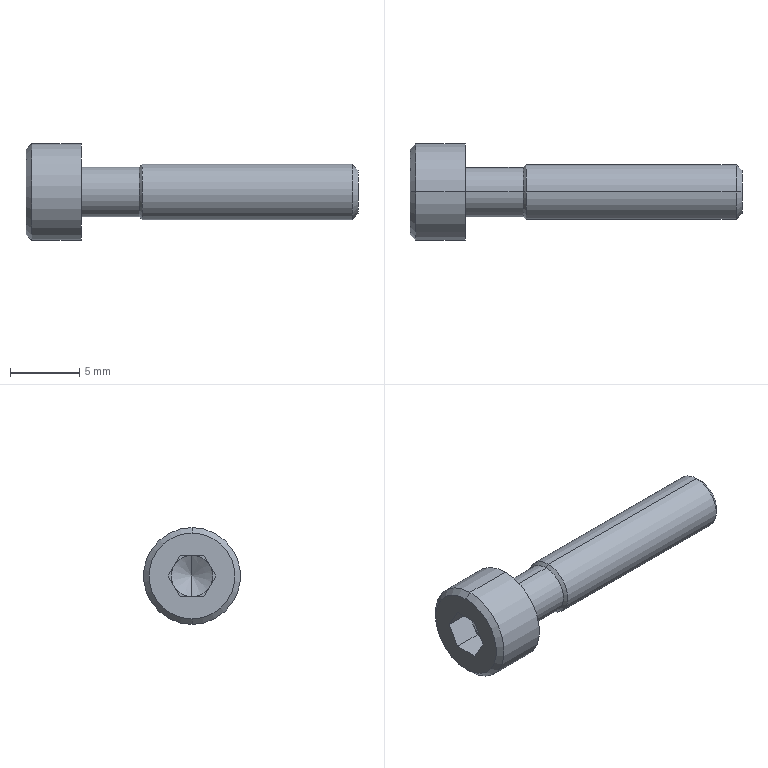Part | STEP file | 0243_Z_SCBS4-20_1 | 1 solid | 29 faces | box 24 x 7 x 7 mm | volume 373.888 mm3 | plane 15 | cone 8 | cylinder 6 | commonest cylinder face diameters 3.57 x2 4 x2 7 x2